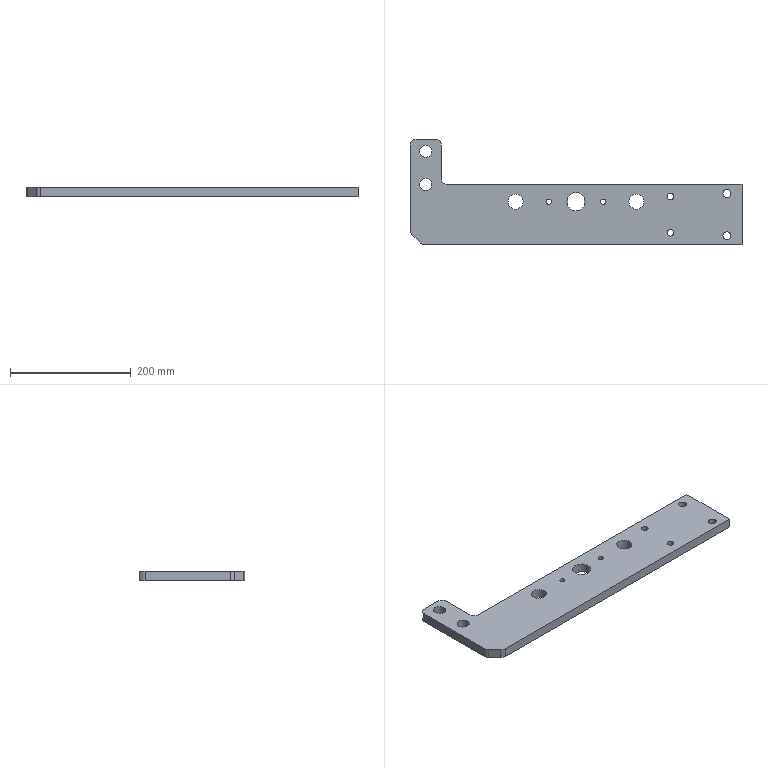Part | STEP file | 1 solid | 40 faces | box 549.959 x 175.002 x 16 mm | volume 892550 mm3 | cylinder 27 | plane 9 | cone 4 | commonest cylinder face diameters 20 x9 8.5 x4 11 x4 13 x4 25 x4 30 x2